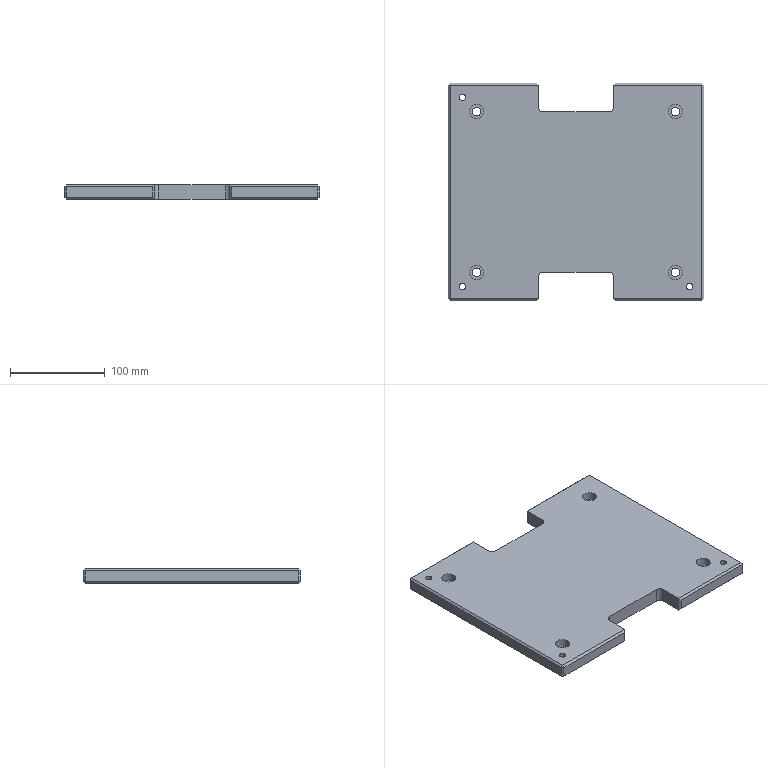Part | STEP file | Fixture base plate | 1 solid | 72 faces | box 270 x 230 x 15 mm | volume 846944 mm3 | plane 46 | cylinder 26 | commonest cylinder face diameters 9 x8 15 x8 6.8 x6 10 x4